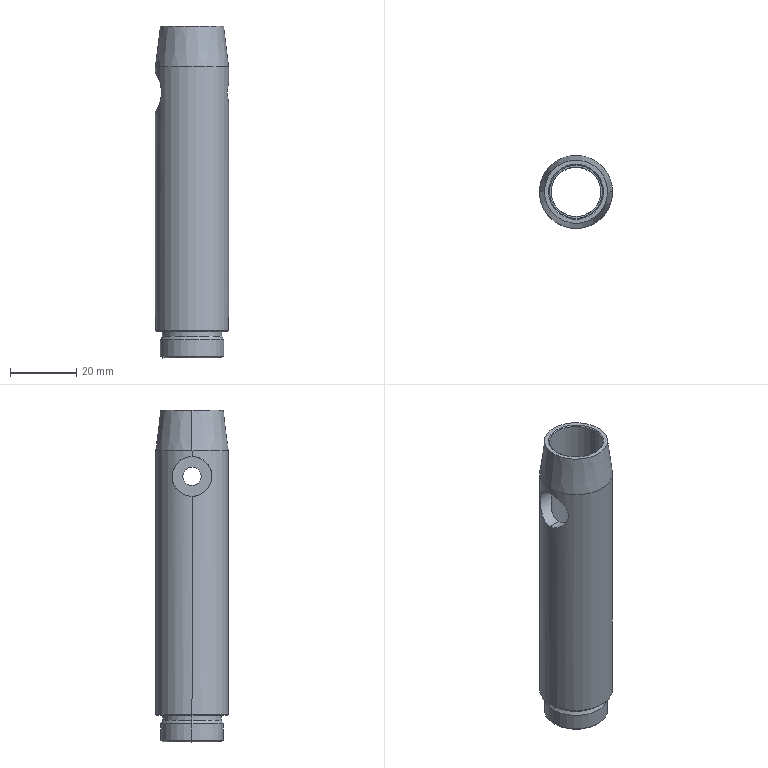Part | SolidWorks | features BaseBody 1 | 1 solid | 36 faces | box 22 x 22 x 100 mm | volume 17628 mm3 | cylinder 18 | cone 12 | plane 6 | commonest cylinder face diameters 12.01 x4 16 x4 5.5 x2 15 x2 17.8 x2 19 x2
STEP:
#1=CARTESIAN_POINT('',(469.537,37.715,-6.334));
#2=VERTEX_POINT('',#1);
#3=CARTESIAN_POINT('',(491.537,37.715,-6.334));
#4=VERTEX_POINT('',#3);
#5=CARTESIAN_POINT('',(480.537,37.715,-6.334));
#6=DIRECTION('',(0.000000013,0.,-1.));
#7=DIRECTION('',(0.,1.,0.));
#8=AXIS2_PLACEMENT_3D('',#5,#6,#7);
#9=CIRCLE('',#8,11.);
#10=EDGE_CURVE('',#2,#4,#9,.T.);
#11=ORIENTED_EDGE('',*,*,#10,.F.);
#12=CARTESIAN_POINT('',(469.537,37.715,59.361));
#13=VERTEX_POINT('',#12);
#14=CARTESIAN_POINT('',(469.537,37.715,-6.334));
#15=DIRECTION('',(-0.000000013,0.,1.));
#16=VECTOR('',#15,1000.);
#17=LINE('',#14,#16);
#18=EDGE_CURVE('',#2,#13,#17,.T.);
#19=ORIENTED_EDGE('',*,*,#18,.T.);
#20=CARTESIAN_POINT('',(469.537,37.715,71.371));
#21=VERTEX_POINT('',#20);
#22=CARTESIAN_POINT('',(469.537,37.715,71.371));
#23=CARTESIAN_POINT('',(469.537,37.916,71.371));
#24=CARTESIAN_POINT('',(469.542,38.12,71.361));
#25=CARTESIAN_POINT('',(469.565,38.52,71.32));
#26=CARTESIAN_POINT('',(469.581,38.717,71.29));
#27=CARTESIAN_POINT('',(469.624,39.107,71.211));
#28=CARTESIAN_POINT('',(469.65,39.3,71.161));
#29=CARTESIAN_POINT('',(469.712,39.68,71.044));
#30=CARTESIAN_POINT('',(469.748,39.868,70.975));
#31=CARTESIAN_POINT('',(469.867,40.414,70.745));
#32=CARTESIAN_POINT('',(469.96,40.756,70.558));
#33=CARTESIAN_POINT('',(470.116,41.24,70.231));
#34=CARTESIAN_POINT('',(470.17,41.397,70.114));
#35=CARTESIAN_POINT('',(470.281,41.695,69.866));
#36=CARTESIAN_POINT('',(470.337,41.837,69.737));
#37=CARTESIAN_POINT('',(470.508,42.243,69.328));
#38=CARTESIAN_POINT('',(470.624,42.488,69.03));
#39=CARTESIAN_POINT('',(470.844,42.921,68.383));
#40=CARTESIAN_POINT('',(470.946,43.104,68.043));
#41=CARTESIAN_POINT('',(471.077,43.33,67.504));
#42=CARTESIAN_POINT('',(471.118,43.396,67.32));
#43=CARTESIAN_POINT('',(471.189,43.513,66.941));
#44=CARTESIAN_POINT('',(471.22,43.562,66.746));
#45=CARTESIAN_POINT('',(471.295,43.681,66.157));
#46=CARTESIAN_POINT('',(471.321,43.721,65.756));
#47=CARTESIAN_POINT('',(471.32,43.719,64.946));
#48=CARTESIAN_POINT('',(471.292,43.677,64.549));
#49=CARTESIAN_POINT('',(471.192,43.518,63.772));
#50=CARTESIAN_POINT('',(471.117,43.398,63.389));
#51=CARTESIAN_POINT('',(470.94,43.094,62.669));
#52=CARTESIAN_POINT('',(470.838,42.909,62.328));
#53=CARTESIAN_POINT('',(470.617,42.474,61.684));
#54=CARTESIAN_POINT('',(470.502,42.229,61.387));
#55=CARTESIAN_POINT('',(470.331,41.822,60.981));
#56=CARTESIAN_POINT('',(470.275,41.68,60.852));
#57=CARTESIAN_POINT('',(470.165,41.381,60.606));
#58=CARTESIAN_POINT('',(470.11,41.224,60.489));
#59=CARTESIAN_POINT('',(469.956,40.741,60.165));
#60=CARTESIAN_POINT('',(469.863,40.4,59.981));
#61=CARTESIAN_POINT('',(469.707,39.678,59.678));
#62=CARTESIAN_POINT('',(469.643,39.292,59.558));
#63=CARTESIAN_POINT('',(469.559,38.512,59.401));
#64=CARTESIAN_POINT('',(469.537,38.117,59.361));
#65=CARTESIAN_POINT('',(469.537,37.715,59.361));
#66=B_SPLINE_CURVE_WITH_KNOTS('',3,(#22,#23,#24,#25,#26,#27,#28,#29,#30,#31,#32,#33,#34,#35,#36,#37,#38,#39,#40,#41,#42,#43,#44,#45,#46,#47,#48,#49,#50,#51,#52,#53,#54,#55,#56,#57,#58,#59,#60,#61,#62,#63,#64,#65),.UNSPECIFIED.,.F.,.F.,(4,2,2,2,2,2,2,2,2,2,2,2,2,2,2,2,2,2,2,2,2,4),(0.02874,0.02934,0.02994,0.03054,0.03113,0.03233,0.03293,0.03353,0.03472,0.03592,0.03652,0.03712,0.03832,0.03951,0.04071,0.04191,0.0431,0.0437,0.0443,0.0455,0.04669,0.04789),.UNSPECIFIED.);
#67=EDGE_CURVE('',#21,#13,#66,.T.);
#68=ORIENTED_EDGE('',*,*,#67,.F.);
#69=CARTESIAN_POINT('',(469.537,37.715,73.266));
#70=VERTEX_POINT('',#69);
#71=CARTESIAN_POINT('',(469.537,37.715,-6.334));
#72=DIRECTION('',(-0.000000013,0.,1.));
#73=VECTOR('',#72,1000.);
#74=LINE('',#71,#73);
#75=EDGE_CURVE('',#21,#70,#74,.T.);
#76=ORIENTED_EDGE('',*,*,#75,.T.);
#77=CARTESIAN_POINT('',(491.537,37.715,73.266));
#78=VERTEX_POINT('',#77);
#79=CARTESIAN_POINT('',(480.537,37.715,73.266));
#80=DIRECTION('',(-0.000000013,0.,1.));
#81=DIRECTION('',(0.,1.,0.));
#82=AXIS2_PLACEMENT_3D('',#79,#80,#81);
#83=CIRCLE('',#82,11.);
#84=EDGE_CURVE('',#78,#70,#83,.T.);
#85=ORIENTED_EDGE('',*,*,#84,.F.);
#86=CARTESIAN_POINT('',(491.537,37.715,68.116));
#87=VERTEX_POINT('',#86);
#88=CARTESIAN_POINT('',(491.537,37.715,-6.334));
#89=DIRECTION('',(-0.000000013,0.,1.));
#90=VECTOR('',#89,1000.);
#91=LINE('',#88,#90);
#92=EDGE_CURVE('',#87,#78,#91,.T.);
#93=ORIENTED_EDGE('',*,*,#92,.F.);
#94=CARTESIAN_POINT('',(491.537,37.715,62.616));
#95=VERTEX_POINT('',#94);
#96=CARTESIAN_POINT('',(491.537,37.715,62.616));
#97=CARTESIAN_POINT('',(491.537,37.895,62.616));
#98=CARTESIAN_POINT('',(491.532,38.078,62.634));
#99=CARTESIAN_POINT('',(491.515,38.431,62.705));
#100=CARTESIAN_POINT('',(491.502,38.603,62.757));
#101=CARTESIAN_POINT('',(491.454,39.103,62.965));
#102=CARTESIAN_POINT('',(491.409,39.406,63.167));
#103=CARTESIAN_POINT('',(491.341,39.787,63.55));
#104=CARTESIAN_POINT('',(491.318,39.901,63.688));
#105=CARTESIAN_POINT('',(491.276,40.1,63.985));
#106=CARTESIAN_POINT('',(491.256,40.186,64.146));
#107=CARTESIAN_POINT('',(491.223,40.324,64.478));
#108=CARTESIAN_POINT('',(491.21,40.376,64.649));
#109=CARTESIAN_POINT('',(491.192,40.447,65.003));
#110=CARTESIAN_POINT('',(491.188,40.465,65.186));
#111=CARTESIAN_POINT('',(491.188,40.465,65.551));
#112=CARTESIAN_POINT('',(491.192,40.446,65.73));
#113=CARTESIAN_POINT('',(491.21,40.376,66.082));
#114=CARTESIAN_POINT('',(491.224,40.322,66.257));
#115=CARTESIAN_POINT('',(491.256,40.184,66.59));
#116=CARTESIAN_POINT('',(491.276,40.099,66.747));
#117=CARTESIAN_POINT('',(491.318,39.9,67.045));
#118=CARTESIAN_POINT('',(491.341,39.784,67.186));
#119=CARTESIAN_POINT('',(491.409,39.405,67.564));
#120=CARTESIAN_POINT('',(491.454,39.099,67.769));
#121=CARTESIAN_POINT('',(491.502,38.603,67.975));
#122=CARTESIAN_POINT('',(491.515,38.429,68.028));
#123=CARTESIAN_POINT('',(491.532,38.074,68.098));
#124=CARTESIAN_POINT('',(491.537,37.895,68.116));
#125=CARTESIAN_POINT('',(491.537,37.715,68.116));
#126=B_SPLINE_CURVE_WITH_KNOTS('',3,(#96,#97,#98,#99,#100,#101,#102,#103,#104,#105,#106,#107,#108,#109,#110,#111,#112,#113,#114,#115,#116,#117,#118,#119,#120,#121,#122,#123,#124,#125),.UNSPECIFIED.,.F.,.F.,(4,2,2,2,2,2,2,2,2,2,2,2,2,2,4),(0.004317,0.004856,0.005396,0.006474,0.007014,0.007553,0.008092,0.008632,0.009171,0.00971,0.01025,0.01079,0.01187,0.01241,0.01295),.UNSPECIFIED.);
#127=EDGE_CURVE('',#95,#87,#126,.T.);
#128=ORIENTED_EDGE('',*,*,#127,.F.);
#129=CARTESIAN_POINT('',(491.537,37.715,-6.334));
#130=DIRECTION('',(-0.000000013,0.,1.));
#131=VECTOR('',#130,1000.);
#132=LINE('',#129,#131);
#133=EDGE_CURVE('',#4,#95,#132,.T.);
#134=ORIENTED_EDGE('',*,*,#133,.F.);
#135=EDGE_LOOP('',(#11,#19,#68,#76,#85,#93,#128,#134));
#136=FACE_OUTER_BOUND('',#135,.T.);
#137=CARTESIAN_POINT('',(480.537,37.715,-6.334));
#138=DIRECTION('',(-0.000000013,0.,1.));
#139=DIRECTION('',(1.,0.,0.000000013));
#140=AXIS2_PLACEMENT_3D('',#137,#138,#139);
#141=CYLINDRICAL_SURFACE('',#140,11.);
#142=ADVANCED_FACE('',(#136),#141,.T.);
#143=CARTESIAN_POINT('',(469.837,37.715,-6.634));
#144=VERTEX_POINT('',#143);
#145=CARTESIAN_POINT('',(491.237,37.715,-6.634));
#146=VERTEX_POINT('',#145);
#147=CARTESIAN_POINT('',(480.537,37.715,-6.634));
#148=DIRECTION('',(0.000000013,0.,-1.));
#149=DIRECTION('',(1.,0.,0.000000013));
#150=AXIS2_PLACEMENT_3D('',#147,#148,#149);
#151=CIRCLE('',#150,10.7);
#152=EDGE_CURVE('',#144,#146,#151,.T.);
#153=ORIENTED_EDGE('',*,*,#152,.F.);
#154=CARTESIAN_POINT('',(469.837,37.715,-6.634));
#155=DIRECTION('',(-0.7071,0.,0.7071));
#156=VECTOR('',#155,1000.);
#157=LINE('',#154,#156);
#158=EDGE_CURVE('',#144,#2,#157,.T.);
#159=ORIENTED_EDGE('',*,*,#158,.T.);
#160=ORIENTED_EDGE('',*,*,#10,.T.);
#161=CARTESIAN_POINT('',(491.237,37.715,-6.634));
#162=DIRECTION('',(0.7071,0.,0.7071));
#163=VECTOR('',#162,1000.);
#164=LINE('',#161,#163);
#165=EDGE_CURVE('',#146,#4,#164,.T.);
#166=ORIENTED_EDGE('',*,*,#165,.F.);
#167=EDGE_LOOP('',(#153,#159,#160,#166));
#168=FACE_OUTER_BOUND('',#167,.T.);
#169=CARTESIAN_POINT('',(480.537,37.715,-6.634));
#170=DIRECTION('',(-0.000000013,0.,1.));
#171=DIRECTION('',(1.,0.,0.000000013));
#172=AXIS2_PLACEMENT_3D('',#169,#170,#171);
#173=CONICAL_SURFACE('',#172,10.7,0.7854);
#174=ADVANCED_FACE('',(#168),#173,.T.);
#175=CARTESIAN_POINT('',(490.037,37.715,85.366));
#176=VERTEX_POINT('',#175);
#177=CARTESIAN_POINT('',(471.037,37.715,85.366));
#178=VERTEX_POINT('',#177);
#179=CARTESIAN_POINT('',(480.537,37.715,85.366));
#180=DIRECTION('',(-0.000000013,0.,1.));
#181=DIRECTION('',(-1.,0.,-0.000000013));
#182=AXIS2_PLACEMENT_3D('',#179,#180,#181);
#183=CIRCLE('',#182,9.5);
#184=EDGE_CURVE('',#176,#178,#183,.T.);
#185=ORIENTED_EDGE('',*,*,#184,.F.);
#186=CARTESIAN_POINT('',(491.537,37.715,73.266));
#187=DIRECTION('',(0.123,0.,-0.9924));
#188=VECTOR('',#187,1000.);
#189=LINE('',#186,#188);
#190=EDGE_CURVE('',#176,#78,#189,.T.);
#191=ORIENTED_EDGE('',*,*,#190,.T.);
#192=ORIENTED_EDGE('',*,*,#84,.T.);
#193=CARTESIAN_POINT('',(469.537,37.715,73.266));
#194=DIRECTION('',(-0.123,0.,-0.9924));
#195=VECTOR('',#194,1000.);
#196=LINE('',#193,#195);
#197=EDGE_CURVE('',#178,#70,#196,.T.);
#198=ORIENTED_EDGE('',*,*,#197,.F.);
#199=EDGE_LOOP('',(#185,#191,#192,#198));
#200=FACE_OUTER_BOUND('',#199,.T.);
#201=CARTESIAN_POINT('',(480.537,37.715,73.266));
#202=DIRECTION('',(0.000000013,0.,-1.));
#203=DIRECTION('',(-1.,0.,-0.000000013));
#204=AXIS2_PLACEMENT_3D('',#201,#202,#203);
#205=CONICAL_SURFACE('',#204,11.,0.1233);
#206=ADVANCED_FACE('',(#200),#205,.T.);
#207=CARTESIAN_POINT('',(491.537,37.715,68.116));
#208=CARTESIAN_POINT('',(491.537,37.535,68.116));
#209=CARTESIAN_POINT('',(491.532,37.352,68.098));
#210=CARTESIAN_POINT('',(491.515,36.998,68.027));
#211=CARTESIAN_POINT('',(491.502,36.827,67.975));
#212=CARTESIAN_POINT('',(491.454,36.326,67.767));
#213=CARTESIAN_POINT('',(491.409,36.024,67.564));
#214=CARTESIAN_POINT('',(491.341,35.642,67.182));
#215=CARTESIAN_POINT('',(491.318,35.529,67.044));
#216=CARTESIAN_POINT('',(491.276,35.33,66.747));
#217=CARTESIAN_POINT('',(491.256,35.244,66.586));
#218=CARTESIAN_POINT('',(491.223,35.106,66.254));
#219=CARTESIAN_POINT('',(491.21,35.054,66.083));
#220=CARTESIAN_POINT('',(491.192,34.983,65.728));
#221=CARTESIAN_POINT('',(491.188,34.965,65.546));
#222=CARTESIAN_POINT('',(491.188,34.965,65.181));
#223=CARTESIAN_POINT('',(491.192,34.983,65.002));
#224=CARTESIAN_POINT('',(491.21,35.054,64.65));
#225=CARTESIAN_POINT('',(491.224,35.107,64.475));
#226=CARTESIAN_POINT('',(491.256,35.245,64.142));
#227=CARTESIAN_POINT('',(491.276,35.33,63.985));
#228=CARTESIAN_POINT('',(491.318,35.53,63.686));
#229=CARTESIAN_POINT('',(491.341,35.646,63.546));
#230=CARTESIAN_POINT('',(491.409,36.025,63.167));
#231=CARTESIAN_POINT('',(491.454,36.33,62.963));
#232=CARTESIAN_POINT('',(491.502,36.826,62.757));
#233=CARTESIAN_POINT('',(491.515,37.,62.704));
#234=CARTESIAN_POINT('',(491.532,37.356,62.633));
#235=CARTESIAN_POINT('',(491.537,37.535,62.616));
#236=CARTESIAN_POINT('',(491.537,37.715,62.616));
#237=B_SPLINE_CURVE_WITH_KNOTS('',3,(#207,#208,#209,#210,#211,#212,#213,#214,#215,#216,#217,#218,#219,#220,#221,#222,#223,#224,#225,#226,#227,#228,#229,#230,#231,#232,#233,#234,#235,#236),.UNSPECIFIED.,.F.,.F.,(4,2,2,2,2,2,2,2,2,2,2,2,2,2,4),(0.01295,0.01349,0.01403,0.0151,0.01564,0.01618,0.01672,0.01726,0.0178,0.01834,0.01888,0.01942,0.0205,0.02104,0.02158),.UNSPECIFIED.);
#238=EDGE_CURVE('',#87,#95,#237,.T.);
#239=ORIENTED_EDGE('',*,*,#238,.T.);
#240=CARTESIAN_POINT('',(489.037,37.715,62.616));
#241=VERTEX_POINT('',#240);
#242=CARTESIAN_POINT('',(491.552,37.715,62.616));
#243=DIRECTION('',(-1.,0.,-0.000000013));
#244=VECTOR('',#243,1000.);
#245=LINE('',#242,#244);
#246=EDGE_CURVE('',#95,#241,#245,.T.);
#247=ORIENTED_EDGE('',*,*,#246,.T.);
#248=CARTESIAN_POINT('',(489.037,37.715,68.116));
#249=VERTEX_POINT('',#248);
#250=CARTESIAN_POINT('',(489.037,37.715,65.366));
#251=DIRECTION('',(-1.,0.,-0.000000013));
#252=DIRECTION('',(-0.000000013,0.,1.));
#253=AXIS2_PLACEMENT_3D('',#250,#251,#252);
#254=CIRCLE('',#253,2.75);
#255=EDGE_CURVE('',#241,#249,#254,.T.);
#256=ORIENTED_EDGE('',*,*,#255,.T.);
#257=CARTESIAN_POINT('',(491.552,37.715,68.116));
#258=DIRECTION('',(-1.,0.,-0.000000013));
#259=VECTOR('',#258,1000.);
#260=LINE('',#257,#259);
#261=EDGE_CURVE('',#87,#249,#260,.T.);
#262=ORIENTED_EDGE('',*,*,#261,.F.);
#263=EDGE_LOOP('',(#239,#247,#256,#262));
#264=FACE_OUTER_BOUND('',#263,.T.);
#265=CARTESIAN_POINT('',(491.552,37.715,65.366));
#266=DIRECTION('',(-1.,0.,-0.000000013));
#267=DIRECTION('',(-0.000000013,0.,1.));
#268=AXIS2_PLACEMENT_3D('',#265,#266,#267);
#269=CYLINDRICAL_SURFACE('',#268,2.75);
#270=ADVANCED_FACE('',(#264),#269,.F.);
#271=CARTESIAN_POINT('',(469.537,37.715,59.361));
#272=CARTESIAN_POINT('',(469.537,37.514,59.361));
#273=CARTESIAN_POINT('',(469.542,37.31,59.371));
#274=CARTESIAN_POINT('',(469.564,36.911,59.412));
#275=CARTESIAN_POINT('',(469.581,36.713,59.442));
#276=CARTESIAN_POINT('',(469.623,36.324,59.521));
#277=CARTESIAN_POINT('',(469.65,36.131,59.57));
#278=CARTESIAN_POINT('',(469.712,35.752,59.687));
#279=CARTESIAN_POINT('',(469.748,35.563,59.756));
#280=CARTESIAN_POINT('',(469.866,35.018,59.986));
#281=CARTESIAN_POINT('',(469.96,34.676,60.172));
#282=CARTESIAN_POINT('',(470.115,34.192,60.499));
#283=CARTESIAN_POINT('',(470.169,34.036,60.616));
#284=CARTESIAN_POINT('',(470.28,33.737,60.863));
#285=CARTESIAN_POINT('',(470.336,33.595,60.992));
#286=CARTESIAN_POINT('',(470.507,33.189,61.4));
#287=CARTESIAN_POINT('',(470.622,32.944,61.698));
#288=CARTESIAN_POINT('',(470.842,32.511,62.344));
#289=CARTESIAN_POINT('',(470.944,32.328,62.684));
#290=CARTESIAN_POINT('',(471.076,32.102,63.221));
#291=CARTESIAN_POINT('',(471.116,32.035,63.405));
#292=CARTESIAN_POINT('',(471.187,31.919,63.783));
#293=CARTESIAN_POINT('',(471.219,31.869,63.978));
#294=CARTESIAN_POINT('',(471.294,31.75,64.566));
#295=CARTESIAN_POINT('',(471.321,31.709,64.965));
#296=CARTESIAN_POINT('',(471.32,31.71,65.777));
#297=CARTESIAN_POINT('',(471.293,31.751,66.174));
#298=CARTESIAN_POINT('',(471.193,31.909,66.952));
#299=CARTESIAN_POINT('',(471.119,32.029,67.336));
#300=CARTESIAN_POINT('',(470.942,32.332,68.057));
#301=CARTESIAN_POINT('',(470.839,32.517,68.398));
#302=CARTESIAN_POINT('',(470.619,32.952,69.044));
#303=CARTESIAN_POINT('',(470.503,33.197,69.341));
#304=CARTESIAN_POINT('',(470.333,33.604,69.748));
#305=CARTESIAN_POINT('',(470.276,33.747,69.877));
#306=CARTESIAN_POINT('',(470.166,34.045,70.123));
#307=CARTESIAN_POINT('',(470.111,34.202,70.241));
#308=CARTESIAN_POINT('',(469.957,34.686,70.566));
#309=CARTESIAN_POINT('',(469.864,35.027,70.75));
#310=CARTESIAN_POINT('',(469.708,35.749,71.054));
#311=CARTESIAN_POINT('',(469.644,36.136,71.173));
#312=CARTESIAN_POINT('',(469.559,36.916,71.331));
#313=CARTESIAN_POINT('',(469.537,37.312,71.371));
#314=CARTESIAN_POINT('',(469.537,37.715,71.371));
#315=B_SPLINE_CURVE_WITH_KNOTS('',3,(#271,#272,#273,#274,#275,#276,#277,#278,#279,#280,#281,#282,#283,#284,#285,#286,#287,#288,#289,#290,#291,#292,#293,#294,#295,#296,#297,#298,#299,#300,#301,#302,#303,#304,#305,#306,#307,#308,#309,#310,#311,#312,#313,#314),.UNSPECIFIED.,.F.,.F.,(4,2,2,2,2,2,2,2,2,2,2,2,2,2,2,2,2,2,2,2,2,4),(0.00959,0.01019,0.01079,0.01139,0.01198,0.01318,0.01378,0.01438,0.01557,0.01677,0.01737,0.01797,0.01917,0.02036,0.02156,0.02276,0.02395,0.02455,0.02515,0.02635,0.02754,0.02874),.UNSPECIFIED.);
#316=EDGE_CURVE('',#13,#21,#315,.T.);
#317=ORIENTED_EDGE('',*,*,#316,.T.);
#318=CARTESIAN_POINT('',(473.037,37.715,71.371));
#319=VERTEX_POINT('',#318);
#320=CARTESIAN_POINT('',(469.498,37.715,71.371));
#321=DIRECTION('',(1.,0.,0.000000013));
#322=VECTOR('',#321,1000.);
#323=LINE('',#320,#322);
#324=EDGE_CURVE('',#21,#319,#323,.T.);
#325=ORIENTED_EDGE('',*,*,#324,.T.);
#326=CARTESIAN_POINT('',(473.037,37.715,59.361));
#327=VERTEX_POINT('',#326);
#328=CARTESIAN_POINT('',(473.037,37.715,71.371));
#329=CARTESIAN_POINT('',(473.037,37.507,71.371));
#330=CARTESIAN_POINT('',(473.045,37.3,71.36));
#331=CARTESIAN_POINT('',(473.08,36.888,71.317));
#332=CARTESIAN_POINT('',(473.106,36.68,71.285));
#333=CARTESIAN_POINT('',(473.207,36.074,71.157));
#334=CARTESIAN_POINT('',(473.305,35.689,71.033));
#335=CARTESIAN_POINT('',(473.491,35.138,70.794));
#336=CARTESIAN_POINT('',(473.559,34.959,70.705));
#337=CARTESIAN_POINT('',(473.704,34.617,70.514));
#338=CARTESIAN_POINT('',(473.781,34.453,70.412));
#339=CARTESIAN_POINT('',(474.023,33.98,70.084));
#340=CARTESIAN_POINT('',(474.202,33.687,69.836));
#341=CARTESIAN_POINT('',(474.567,33.163,69.301));
#342=CARTESIAN_POINT('',(474.755,32.929,69.013));
#343=CARTESIAN_POINT('',(475.127,32.513,68.39));
#344=CARTESIAN_POINT('',(475.309,32.333,68.057));
#345=CARTESIAN_POINT('',(475.553,32.109,67.528));
#346=CARTESIAN_POINT('',(475.629,32.042,67.347));
#347=CARTESIAN_POINT('',(475.769,31.925,66.97));
#348=CARTESIAN_POINT('',(475.832,31.874,66.774));
#349=CARTESIAN_POINT('',(475.986,31.752,66.181));
#350=CARTESIAN_POINT('',(476.045,31.709,65.771));
#351=CARTESIAN_POINT('',(476.042,31.711,64.929));
#352=CARTESIAN_POINT('',(475.981,31.756,64.521));
#353=CARTESIAN_POINT('',(475.822,31.881,63.926));
#354=CARTESIAN_POINT('',(475.759,31.933,63.732));
#355=CARTESIAN_POINT('',(475.619,32.051,63.36));
#356=CARTESIAN_POINT('',(475.542,32.119,63.18));
#357=CARTESIAN_POINT('',(475.297,32.344,62.653));
#358=CARTESIAN_POINT('',(475.114,32.526,62.32));
#359=CARTESIAN_POINT('',(474.746,32.941,61.704));
#360=CARTESIAN_POINT('',(474.559,33.174,61.419));
#361=CARTESIAN_POINT('',(474.196,33.697,60.888));
#362=CARTESIAN_POINT('',(474.018,33.989,60.641));
#363=CARTESIAN_POINT('',(473.696,34.619,60.206));
#364=CARTESIAN_POINT('',(473.552,34.957,60.017));
#365=CARTESIAN_POINT('',(473.367,35.506,59.778));
#366=CARTESIAN_POINT('',(473.311,35.696,59.707));
#367=CARTESIAN_POINT('',(473.214,36.082,59.584));
#368=CARTESIAN_POINT('',(473.173,36.278,59.532));
#369=CARTESIAN_POINT('',(473.073,36.879,59.405));
#370=CARTESIAN_POINT('',(473.037,37.3,59.361));
#371=CARTESIAN_POINT('',(473.037,37.715,59.361));
#372=B_SPLINE_CURVE_WITH_KNOTS('',3,(#328,#329,#330,#331,#332,#333,#334,#335,#336,#337,#338,#339,#340,#341,#342,#343,#344,#345,#346,#347,#348,#349,#350,#351,#352,#353,#354,#355,#356,#357,#358,#359,#360,#361,#362,#363,#364,#365,#366,#367,#368,#369,#370,#371),.UNSPECIFIED.,.F.,.F.,(4,2,2,2,2,2,2,2,2,2,2,2,2,2,2,2,2,2,2,2,2,4),(0.02988,0.0305,0.03112,0.03237,0.03299,0.03361,0.03485,0.0361,0.03734,0.03796,0.03859,0.03983,0.04107,0.0417,0.04232,0.04356,0.04481,0.04605,0.0473,0.04792,0.04854,0.04978),.UNSPECIFIED.);
#373=EDGE_CURVE('',#319,#327,#372,.T.);
#374=ORIENTED_EDGE('',*,*,#373,.T.);
#375=CARTESIAN_POINT('',(469.498,37.715,59.361));
#376=DIRECTION('',(1.,0.,0.000000013));
#377=VECTOR('',#376,1000.);
#378=LINE('',#375,#377);
#379=EDGE_CURVE('',#13,#327,#378,.T.);
#380=ORIENTED_EDGE('',*,*,#379,.F.);
#381=EDGE_LOOP('',(#317,#325,#374,#380));
#382=FACE_OUTER_BOUND('',#381,.T.);
#383=CARTESIAN_POINT('',(469.498,37.715,65.366));
#384=DIRECTION('',(1.,0.,0.000000013));
#385=DIRECTION('',(0.000000013,0.,-1.));
#386=AXIS2_PLACEMENT_3D('',#383,#384,#385);
#387=CYLINDRICAL_SURFACE('',#386,6.005);
#388=ADVANCED_FACE('',(#382),#387,.F.);
#389=CARTESIAN_POINT('',(488.037,37.715,-2.634));
#390=VERTEX_POINT('',#389);
#391=CARTESIAN_POINT('',(473.037,37.715,-2.634));
#392=VERTEX_POINT('',#391);
#393=CARTESIAN_POINT('',(480.537,37.715,-2.634));
#394=DIRECTION('',(0.000000013,0.,-1.));
#395=DIRECTION('',(1.,0.,0.000000013));
#396=AXIS2_PLACEMENT_3D('',#393,#394,#395);
#397=CIRCLE('',#396,7.5);
#398=EDGE_CURVE('',#390,#392,#397,.T.);
#399=ORIENTED_EDGE('',*,*,#398,.T.);
#400=CARTESIAN_POINT('',(473.037,37.715,-2.634));
#401=DIRECTION('',(-0.000000013,0.,1.));
#402=VECTOR('',#401,1000.);
#403=LINE('',#400,#402);
#404=EDGE_CURVE('',#392,#327,#403,.T.);
#405=ORIENTED_EDGE('',*,*,#404,.T.);
#406=ORIENTED_EDGE('',*,*,#373,.F.);
#407=CARTESIAN_POINT('',(473.037,37.715,73.366));
#408=VERTEX_POINT('',#407);
#409=CARTESIAN_POINT('',(473.037,37.715,-2.634));
#410=DIRECTION('',(-0.000000013,0.,1.));
#411=VECTOR('',#410,1000.);
#412=LINE('',#409,#411);
#413=EDGE_CURVE('',#319,#408,#412,.T.);
#414=ORIENTED_EDGE('',*,*,#413,.T.);
#415=CARTESIAN_POINT('',(488.037,37.715,73.366));
#416=VERTEX_POINT('',#415);
#417=CARTESIAN_POINT('',(480.537,37.715,73.366));
#418=DIRECTION('',(-0.000000013,0.,1.));
#419=DIRECTION('',(1.,0.,0.000000013));
#420=AXIS2_PLACEMENT_3D('',#417,#418,#419);
#421=CIRCLE('',#420,7.5);
#422=EDGE_CURVE('',#408,#416,#421,.T.);
#423=ORIENTED_EDGE('',*,*,#422,.T.);
#424=CARTESIAN_POINT('',(488.037,37.715,71.371));
#425=VERTEX_POINT('',#424);
#426=CARTESIAN_POINT('',(488.037,37.715,-2.634));
#427=DIRECTION('',(-0.000000013,0.,1.));
#428=VECTOR('',#427,1000.);
#429=LINE('',#426,#428);
#430=EDGE_CURVE('',#425,#416,#429,.T.);
#431=ORIENTED_EDGE('',*,*,#430,.F.);
#432=CARTESIAN_POINT('',(488.037,37.715,59.361));
#433=VERTEX_POINT('',#432);
#434=CARTESIAN_POINT('',(488.037,37.715,59.361));
#435=CARTESIAN_POINT('',(488.037,37.508,59.361));
#436=CARTESIAN_POINT('',(488.028,37.301,59.372));
#437=CARTESIAN_POINT('',(487.994,36.889,59.414));
#438=CARTESIAN_POINT('',(487.968,36.682,59.447));
#439=CARTESIAN_POINT('',(487.867,36.077,59.574));
#440=CARTESIAN_POINT('',(487.769,35.692,59.698));
#441=CARTESIAN_POINT('',(487.584,35.142,59.936));
#442=CARTESIAN_POINT('',(487.517,34.964,60.025));
#443=CARTESIAN_POINT('',(487.372,34.623,60.215));
#444=CARTESIAN_POINT('',(487.296,34.459,60.317));
#445=CARTESIAN_POINT('',(487.054,33.986,60.644));
#446=CARTESIAN_POINT('',(486.876,33.693,60.891));
#447=CARTESIAN_POINT('',(486.511,33.169,61.424));
#448=CARTESIAN_POINT('',(486.324,32.936,61.711));
#449=CARTESIAN_POINT('',(485.953,32.519,62.332));
#450=CARTESIAN_POINT('',(485.771,32.338,62.664));
#451=CARTESIAN_POINT('',(485.526,32.114,63.191));
#452=CARTESIAN_POINT('',(485.45,32.047,63.372));
#453=CARTESIAN_POINT('',(485.31,31.929,63.747));
#454=CARTESIAN_POINT('',(485.247,31.877,63.942));
#455=CARTESIAN_POINT('',(485.091,31.754,64.533));
#456=CARTESIAN_POINT('',(485.031,31.71,64.94));
#457=CARTESIAN_POINT('',(485.03,31.709,65.785));
#458=CARTESIAN_POINT('',(485.09,31.753,66.194));
#459=CARTESIAN_POINT('',(485.247,31.878,66.791));
#460=CARTESIAN_POINT('',(485.31,31.929,66.985));
#461=CARTESIAN_POINT('',(485.449,32.047,67.359));
#462=CARTESIAN_POINT('',(485.526,32.114,67.54));
#463=CARTESIAN_POINT('',(485.77,32.338,68.067));
#464=CARTESIAN_POINT('',(485.954,32.52,68.402));
#465=CARTESIAN_POINT('',(486.323,32.935,69.02));
#466=CARTESIAN_POINT('',(486.51,33.168,69.306));
#467=CARTESIAN_POINT('',(486.874,33.691,69.839));
#468=CARTESIAN_POINT('',(487.052,33.983,70.086));
#469=CARTESIAN_POINT('',(487.375,34.614,70.523));
#470=CARTESIAN_POINT('',(487.52,34.952,70.713));
#471=CARTESIAN_POINT('',(487.706,35.502,70.952));
#472=CARTESIAN_POINT('',(487.762,35.693,71.024));
#473=CARTESIAN_POINT('',(487.859,36.079,71.147));
#474=CARTESIAN_POINT('',(487.9,36.275,71.2));
#475=CARTESIAN_POINT('',(488.001,36.877,71.326));
#476=CARTESIAN_POINT('',(488.037,37.3,71.371));
#477=CARTESIAN_POINT('',(488.037,37.715,71.371));
#478=B_SPLINE_CURVE_WITH_KNOTS('',3,(#434,#435,#436,#437,#438,#439,#440,#441,#442,#443,#444,#445,#446,#447,#448,#449,#450,#451,#452,#453,#454,#455,#456,#457,#458,#459,#460,#461,#462,#463,#464,#465,#466,#467,#468,#469,#470,#471,#472,#473,#474,#475,#476,#477),.UNSPECIFIED.,.F.,.F.,(4,2,2,2,2,2,2,2,2,2,2,2,2,2,2,2,2,2,2,2,2,4),(0.009969,0.01059,0.01121,0.01246,0.01308,0.0137,0.01495,0.01619,0.01743,0.01806,0.01868,0.01992,0.02117,0.02179,0.02241,0.02366,0.0249,0.02614,0.02739,0.02801,0.02863,0.02988),.UNSPECIFIED.);
#479=EDGE_CURVE('',#433,#425,#478,.T.);
#480=ORIENTED_EDGE('',*,*,#479,.F.);
#481=CARTESIAN_POINT('',(488.037,37.715,-2.634));
#482=DIRECTION('',(-0.000000013,0.,1.));
#483=VECTOR('',#482,1000.);
#484=LINE('',#481,#483);
#485=EDGE_CURVE('',#390,#433,#484,.T.);
#486=ORIENTED_EDGE('',*,*,#485,.F.);
#487=EDGE_LOOP('',(#399,#405,#406,#414,#423,#431,#480,#486));
#488=FACE_OUTER_BOUND('',#487,.T.);
#489=CARTESIAN_POINT('',(480.537,37.715,-2.634));
#490=DIRECTION('',(-0.000000013,0.,1.));
#491=DIRECTION('',(1.,0.,0.000000013));
#492=AXIS2_PLACEMENT_3D('',#489,#490,#491);
#493=CYLINDRICAL_SURFACE('',#492,7.5);
#494=ADVANCED_FACE('',(#488),#493,.F.);
#495=CARTESIAN_POINT('',(471.637,37.715,-8.134));
#496=VERTEX_POINT('',#495);
#497=CARTESIAN_POINT('',(489.437,37.715,-8.134));
#498=VERTEX_POINT('',#497);
#499=CARTESIAN_POINT('',(480.537,37.715,-8.134));
#500=DIRECTION('',(0.000000013,0.,-1.));
#501=DIRECTION('',(0.,1.,0.));
#502=AXIS2_PLACEMENT_3D('',#499,#500,#501);
#503=CIRCLE('',#502,8.9);
#504=EDGE_CURVE('',#496,#498,#503,.T.);
#505=ORIENTED_EDGE('',*,*,#504,.F.);
#506=CARTESIAN_POINT('',(471.637,37.715,-6.634));
#507=VERTEX_POINT('',#506);
#508=CARTESIAN_POINT('',(471.637,37.715,-8.134));
#509=DIRECTION('',(-0.000000013,0.,1.));
#510=VECTOR('',#509,1000.);
#511=LINE('',#508,#510);
#512=EDGE_CURVE('',#496,#507,#511,.T.);
#513=ORIENTED_EDGE('',*,*,#512,.T.);
#514=CARTESIAN_POINT('',(489.437,37.715,-6.634));
#515=VERTEX_POINT('',#514);
#516=CARTESIAN_POINT('',(480.537,37.715,-6.634));
#517=DIRECTION('',(0.000000013,0.,-1.));
#518=DIRECTION('',(1.,0.,0.000000013));
#519=AXIS2_PLACEMENT_3D('',#516,#517,#518);
#520=CIRCLE('',#519,8.9);
#521=EDGE_CURVE('',#507,#515,#520,.T.);
#522=ORIENTED_EDGE('',*,*,#521,.T.);
#523=CARTESIAN_POINT('',(489.437,37.715,-8.134));
#524=DIRECTION('',(-0.000000013,0.,1.));
#525=VECTOR('',#524,1000.);
#526=LINE('',#523,#525);
#527=EDGE_CURVE('',#498,#515,#526,.T.);
#528=ORIENTED_EDGE('',*,*,#527,.F.);
#529=EDGE_LOOP('',(#505,#513,#522,#528));
#530=FACE_OUTER_BOUND('',#529,.T.);
#531=CARTESIAN_POINT('',(480.537,37.715,-8.134));
#532=DIRECTION('',(-0.000000013,0.,1.));
#533=DIRECTION('',(1.,0.,0.000000013));
#534=AXIS2_PLACEMENT_3D('',#531,#532,#533);
#535=CYLINDRICAL_SURFACE('',#534,8.9);
#536=ADVANCED_FACE('',(#530),#535,.T.);
#537=CARTESIAN_POINT('',(488.537,37.715,85.066));
#538=VERTEX_POINT('',#537);
#539=CARTESIAN_POINT('',(472.537,37.715,85.066));
#540=VERTEX_POINT('',#539);
#541=CARTESIAN_POINT('',(480.537,37.715,85.066));
#542=DIRECTION('',(0.000000013,0.,-1.));
#543=DIRECTION('',(0.,1.,0.));
#544=AXIS2_PLACEMENT_3D('',#541,#542,#543);
#545=CIRCLE('',#544,8.);
#546=EDGE_CURVE('',#538,#540,#545,.T.);
#547=ORIENTED_EDGE('',*,*,#546,.T.);
#548=CARTESIAN_POINT('',(472.237,37.715,85.366));
#549=VERTEX_POINT('',#548);
#550=CARTESIAN_POINT('',(472.537,37.715,85.066));
#551=DIRECTION('',(-0.7071,0.,0.7071));
#552=VECTOR('',#551,1000.);
#553=LINE('',#550,#552);
#554=EDGE_CURVE('',#540,#549,#553,.T.);
#555=ORIENTED_EDGE('',*,*,#554,.T.);
#556=CARTESIAN_POINT('',(488.837,37.715,85.366));
#557=VERTEX_POINT('',#556);
#558=CARTESIAN_POINT('',(480.537,37.715,85.366));
#559=DIRECTION('',(0.000000013,0.,-1.));
#560=DIRECTION('',(1.,0.,0.000000013));
#561=AXIS2_PLACEMENT_3D('',#558,#559,#560);
#562=CIRCLE('',#561,8.3);
#563=EDGE_CURVE('',#557,#549,#562,.T.);
#564=ORIENTED_EDGE('',*,*,#563,.F.);
#565=CARTESIAN_POINT('',(488.537,37.715,85.066));
#566=DIRECTION('',(0.7071,0.,0.7071));
#567=VECTOR('',#566,1000.);
#568=LINE('',#565,#567);
#569=EDGE_CURVE('',#538,#557,#568,.T.);
#570=ORIENTED_EDGE('',*,*,#569,.F.);
#571=EDGE_LOOP('',(#547,#555,#564,#570));
#572=FACE_OUTER_BOUND('',#571,.T.);
#573=CARTESIAN_POINT('',(480.537,37.715,85.066));
#574=DIRECTION('',(-0.000000013,0.,1.));
#575=DIRECTION('',(1.,0.,0.000000013));
#576=AXIS2_PLACEMENT_3D('',#573,#574,#575);
#577=CONICAL_SURFACE('',#576,8.,0.7854);
#578=ADVANCED_FACE('',(#572),#577,.F.);
#579=ORIENTED_EDGE('',*,*,#479,.T.);
#580=CARTESIAN_POINT('',(489.037,37.715,71.371));
#581=VERTEX_POINT('',#580);
#582=CARTESIAN_POINT('',(485.006,37.715,71.371));
#583=DIRECTION('',(1.,0.,0.000000013));
#584=VECTOR('',#583,1000.);
#585=LINE('',#582,#584);
#586=EDGE_CURVE('',#425,#581,#585,.T.);
#587=ORIENTED_EDGE('',*,*,#586,.T.);
#588=CARTESIAN_POINT('',(489.037,37.715,59.361));
#589=VERTEX_POINT('',#588);
#590=CARTESIAN_POINT('',(489.037,37.715,65.366));
#591=DIRECTION('',(1.,0.,0.000000013));
#592=DIRECTION('',(0.000000013,0.,-1.));
#593=AXIS2_PLACEMENT_3D('',#590,#591,#592);
#594=CIRCLE('',#593,6.005);
#595=EDGE_CURVE('',#581,#589,#594,.T.);
#596=ORIENTED_EDGE('',*,*,#595,.T.);
#597=CARTESIAN_POINT('',(485.006,37.715,59.361));
#598=DIRECTION('',(1.,0.,0.000000013));
#599=VECTOR('',#598,1000.);
#600=LINE('',#597,#599);
#601=EDGE_CURVE('',#433,#589,#600,.T.);
#602=ORIENTED_EDGE('',*,*,#601,.F.);
#603=EDGE_LOOP('',(#579,#587,#596,#602));
#604=FACE_OUTER_BOUND('',#603,.T.);
#605=CARTESIAN_POINT('',(485.006,37.715,65.366));
#606=DIRECTION('',(1.,0.,0.000000013));
#607=DIRECTION('',(0.000000013,0.,-1.));
#608=AXIS2_PLACEMENT_3D('',#605,#606,#607);
#609=CYLINDRICAL_SURFACE('',#608,6.005);
#610=ADVANCED_FACE('',(#604),#609,.F.);
#611=ORIENTED_EDGE('',*,*,#504,.T.);
#612=CARTESIAN_POINT('',(490.037,37.715,-9.173));
#613=VERTEX_POINT('',#612);
#614=CARTESIAN_POINT('',(490.037,37.715,-9.173));
#615=DIRECTION('',(0.5,0.,-0.866));
#616=VECTOR('',#615,1000.);
#617=LINE('',#614,#616);
#618=EDGE_CURVE('',#498,#613,#617,.T.);
#619=ORIENTED_EDGE('',*,*,#618,.T.);
#620=CARTESIAN_POINT('',(471.037,37.715,-9.173));
#621=VERTEX_POINT('',#620);
#622=CARTESIAN_POINT('',(480.537,37.715,-9.173));
#623=DIRECTION('',(0.000000013,0.,-1.));
#624=DIRECTION('',(0.,1.,0.));
#625=AXIS2_PLACEMENT_3D('',#622,#623,#624);
#626=CIRCLE('',#625,9.5);
#627=EDGE_CURVE('',#621,#613,#626,.T.);
#628=ORIENTED_EDGE('',*,*,#627,.F.);
#629=CARTESIAN_POINT('',(471.037,37.715,-9.173));
#630=DIRECTION('',(-0.5,0.,-0.866));
#631=VECTOR('',#630,1000.);
#632=LINE('',#629,#631);
#633=EDGE_CURVE('',#496,#621,#632,.T.);
#634=ORIENTED_EDGE('',*,*,#633,.F.);
#635=EDGE_LOOP('',(#611,#619,#628,#634));
#636=FACE_OUTER_BOUND('',#635,.T.);
#637=CARTESIAN_POINT('',(480.537,37.715,-9.173));
#638=DIRECTION('',(0.000000013,0.,-1.));
#639=DIRECTION('',(-1.,0.,-0.000000013));
#640=AXIS2_PLACEMENT_3D('',#637,#638,#639);
#641=CONICAL_SURFACE('',#640,9.5,0.5236);
#642=ADVANCED_FACE('',(#636),#641,.T.);
#643=CARTESIAN_POINT('',(472.537,37.715,73.366));
#644=VERTEX_POINT('',#643);
#645=CARTESIAN_POINT('',(488.537,37.715,73.366));
#646=VERTEX_POINT('',#645);
#647=CARTESIAN_POINT('',(480.537,37.715,73.366));
#648=DIRECTION('',(-0.000000013,0.,1.));
#649=DIRECTION('',(1.,0.,0.000000013));
#650=AXIS2_PLACEMENT_3D('',#647,#648,#649);
#651=CIRCLE('',#650,8.);
#652=EDGE_CURVE('',#644,#646,#651,.T.);
#653=ORIENTED_EDGE('',*,*,#652,.F.);
#654=CARTESIAN_POINT('',(472.537,37.715,73.366));
#655=DIRECTION('',(-0.000000013,0.,1.));
#656=VECTOR('',#655,1000.);
#657=LINE('',#654,#656);
#658=EDGE_CURVE('',#644,#540,#657,.T.);
#659=ORIENTED_EDGE('',*,*,#658,.T.);
#660=ORIENTED_EDGE('',*,*,#546,.F.);
#661=CARTESIAN_POINT('',(488.537,37.715,73.366));
#662=DIRECTION('',(-0.000000013,0.,1.));
#663=VECTOR('',#662,1000.);
#664=LINE('',#661,#663);
#665=EDGE_CURVE('',#646,#538,#664,.T.);
#666=ORIENTED_EDGE('',*,*,#665,.F.);
#667=EDGE_LOOP('',(#653,#659,#660,#666));
#668=FACE_OUTER_BOUND('',#667,.T.);
#669=CARTESIAN_POINT('',(480.537,37.715,73.366));
#670=DIRECTION('',(-0.000000013,0.,1.));
#671=DIRECTION('',(1.,0.,0.000000013));
#672=AXIS2_PLACEMENT_3D('',#669,#670,#671);
#673=CYLINDRICAL_SURFACE('',#672,8.);
#674=ADVANCED_FACE('',(#668),#673,.F.);
#675=CARTESIAN_POINT('',(488.537,37.715,-14.134));
#676=VERTEX_POINT('',#675);
#677=CARTESIAN_POINT('',(472.537,37.715,-14.134));
#678=VERTEX_POINT('',#677);
#679=CARTESIAN_POINT('',(480.537,37.715,-14.134));
#680=DIRECTION('',(0.000000013,0.,-1.));
#681=DIRECTION('',(0.,1.,0.));
#682=AXIS2_PLACEMENT_3D('',#679,#680,#681);
#683=CIRCLE('',#682,8.);
#684=EDGE_CURVE('',#676,#678,#683,.T.);
#685=ORIENTED_EDGE('',*,*,#684,.T.);
#686=CARTESIAN_POINT('',(472.537,37.715,-2.634));
#687=VERTEX_POINT('',#686);
#688=CARTESIAN_POINT('',(472.537,37.715,-14.134));
#689=DIRECTION('',(-0.000000013,0.,1.));
#690=VECTOR('',#689,1000.);
#691=LINE('',#688,#690);
#692=EDGE_CURVE('',#678,#687,#691,.T.);
#693=ORIENTED_EDGE('',*,*,#692,.T.);
#694=CARTESIAN_POINT('',(488.537,37.715,-2.634));
#695=VERTEX_POINT('',#694);
#696=CARTESIAN_POINT('',(480.537,37.715,-2.634));
#697=DIRECTION('',(-0.000000013,0.,1.));
#698=DIRECTION('',(1.,0.,0.000000013));
#699=AXIS2_PLACEMENT_3D('',#696,#697,#698);
#700=CIRCLE('',#699,8.);
#701=EDGE_CURVE('',#687,#695,#700,.T.);
#702=ORIENTED_EDGE('',*,*,#701,.T.);
#703=CARTESIAN_POINT('',(488.537,37.715,-14.134));
#704=DIRECTION('',(-0.000000013,0.,1.));
#705=VECTOR('',#704,1000.);
#706=LINE('',#703,#705);
#707=EDGE_CURVE('',#676,#695,#706,.T.);
#708=ORIENTED_EDGE('',*,*,#707,.F.);
#709=EDGE_LOOP('',(#685,#693,#702,#708));
#710=FACE_OUTER_BOUND('',#709,.T.);
#711=CARTESIAN_POINT('',(480.537,37.715,-14.134));
#712=DIRECTION('',(-0.000000013,0.,1.));
#713=DIRECTION('',(1.,0.,0.000000013));
#714=AXIS2_PLACEMENT_3D('',#711,#712,#713);
#715=CYLINDRICAL_SURFACE('',#714,8.);
#716=ADVANCED_FACE('',(#710),#715,.F.);
#717=CARTESIAN_POINT('',(471.037,37.715,-14.134));
#718=VERTEX_POINT('',#717);
#719=CARTESIAN_POINT('',(490.037,37.715,-14.134));
#720=VERTEX_POINT('',#719);
#721=CARTESIAN_POINT('',(480.537,37.715,-14.134));
#722=DIRECTION('',(0.000000013,0.,-1.));
#723=DIRECTION('',(0.,1.,0.));
#724=AXIS2_PLACEMENT_3D('',#721,#722,#723);
#725=CIRCLE('',#724,9.5);
#726=EDGE_CURVE('',#718,#720,#725,.T.);
#727=ORIENTED_EDGE('',*,*,#726,.F.);
#728=CARTESIAN_POINT('',(471.037,37.715,-14.134));
#729=DIRECTION('',(-0.000000013,0.,1.));
#730=VECTOR('',#729,1000.);
#731=LINE('',#728,#730);
#732=EDGE_CURVE('',#718,#621,#731,.T.);
#733=ORIENTED_EDGE('',*,*,#732,.T.);
#734=ORIENTED_EDGE('',*,*,#627,.T.);
#735=CARTESIAN_POINT('',(490.037,37.715,-14.134));
#736=DIRECTION('',(-0.000000013,0.,1.));
#737=VECTOR('',#736,1000.);
#738=LINE('',#735,#737);
#739=EDGE_CURVE('',#720,#613,#738,.T.);
#740=ORIENTED_EDGE('',*,*,#739,.F.);
#741=EDGE_LOOP('',(#727,#733,#734,#740));
#742=FACE_OUTER_BOUND('',#741,.T.);
#743=CARTESIAN_POINT('',(480.537,37.715,-14.134));
#744=DIRECTION('',(-0.000000013,0.,1.));
#745=DIRECTION('',(1.,0.,0.000000013));
#746=AXIS2_PLACEMENT_3D('',#743,#744,#745);
#747=CYLINDRICAL_SURFACE('',#746,9.5);
#748=ADVANCED_FACE('',(#742),#747,.T.);
#749=ORIENTED_EDGE('',*,*,#684,.F.);
#750=CARTESIAN_POINT('',(489.037,37.715,-14.634));
#751=VERTEX_POINT('',#750);
#752=CARTESIAN_POINT('',(489.037,37.715,-14.634));
#753=DIRECTION('',(0.7071,0.,-0.7071));
#754=VECTOR('',#753,1000.);
#755=LINE('',#752,#754);
#756=EDGE_CURVE('',#676,#751,#755,.T.);
#757=ORIENTED_EDGE('',*,*,#756,.T.);
#758=CARTESIAN_POINT('',(472.037,37.715,-14.634));
#759=VERTEX_POINT('',#758);
#760=CARTESIAN_POINT('',(480.537,37.715,-14.634));
#761=DIRECTION('',(0.000000013,0.,-1.));
#762=DIRECTION('',(-1.,0.,-0.000000013));
#763=AXIS2_PLACEMENT_3D('',#760,#761,#762);
#764=CIRCLE('',#763,8.5);
#765=EDGE_CURVE('',#751,#759,#764,.T.);
#766=ORIENTED_EDGE('',*,*,#765,.T.);
#767=CARTESIAN_POINT('',(472.037,37.715,-14.634));
#768=DIRECTION('',(-0.7071,0.,-0.7071));
#769=VECTOR('',#768,1000.);
#770=LINE('',#767,#769);
#771=EDGE_CURVE('',#678,#759,#770,.T.);
#772=ORIENTED_EDGE('',*,*,#771,.F.);
#773=EDGE_LOOP('',(#749,#757,#766,#772));
#774=FACE_OUTER_BOUND('',#773,.T.);
#775=CARTESIAN_POINT('',(480.537,37.715,-14.634));
#776=DIRECTION('',(0.000000013,0.,-1.));
#777=DIRECTION('',(-1.,0.,-0.000000013));
#778=AXIS2_PLACEMENT_3D('',#775,#776,#777);
#779=CONICAL_SURFACE('',#778,8.5,0.7854);
#780=ADVANCED_FACE('',(#774),#779,.F.);
#781=CARTESIAN_POINT('',(471.537,37.715,-14.634));
#782=VERTEX_POINT('',#781);
#783=CARTESIAN_POINT('',(489.537,37.715,-14.634));
#784=VERTEX_POINT('',#783);
#785=CARTESIAN_POINT('',(480.537,37.715,-14.634));
#786=DIRECTION('',(0.000000013,0.,-1.));
#787=DIRECTION('',(1.,0.,0.000000013));
#788=AXIS2_PLACEMENT_3D('',#785,#786,#787);
#789=CIRCLE('',#788,9.);
#790=EDGE_CURVE('',#782,#784,#789,.T.);
#791=ORIENTED_EDGE('',*,*,#790,.F.);
#792=CARTESIAN_POINT('',(471.537,37.715,-14.634));
#793=DIRECTION('',(-0.7071,0.,0.7071));
#794=VECTOR('',#793,1000.);
#795=LINE('',#792,#794);
#796=EDGE_CURVE('',#782,#718,#795,.T.);
#797=ORIENTED_EDGE('',*,*,#796,.T.);
#798=ORIENTED_EDGE('',*,*,#726,.T.);
#799=CARTESIAN_POINT('',(489.537,37.715,-14.634));
#800=DIRECTION('',(0.7071,0.,0.7071));
#801=VECTOR('',#800,1000.);
#802=LINE('',#799,#801);
#803=EDGE_CURVE('',#784,#720,#802,.T.);
#804=ORIENTED_EDGE('',*,*,#803,.F.);
#805=EDGE_LOOP('',(#791,#797,#798,#804));
#806=FACE_OUTER_BOUND('',#805,.T.);
#807=CARTESIAN_POINT('',(480.537,37.715,-14.634));
#808=DIRECTION('',(-0.000000013,0.,1.));
#809=DIRECTION('',(1.,0.,0.000000013));
#810=AXIS2_PLACEMENT_3D('',#807,#808,#809);
#811=CONICAL_SURFACE('',#810,9.,0.7854);
#812=ADVANCED_FACE('',(#806),#811,.T.);
#813=ORIENTED_EDGE('',*,*,#18,.F.);
#814=CARTESIAN_POINT('',(480.537,37.715,-6.334));
#815=DIRECTION('',(0.000000013,0.,-1.));
#816=DIRECTION('',(0.,1.,0.));
#817=AXIS2_PLACEMENT_3D('',#814,#815,#816);
#818=CIRCLE('',#817,11.);
#819=EDGE_CURVE('',#4,#2,#818,.T.);
#820=ORIENTED_EDGE('',*,*,#819,.F.);
#821=ORIENTED_EDGE('',*,*,#133,.T.);
#822=ORIENTED_EDGE('',*,*,#238,.F.);
#823=ORIENTED_EDGE('',*,*,#92,.T.);
#824=CARTESIAN_POINT('',(480.537,37.715,73.266));
#825=DIRECTION('',(-0.000000013,0.,1.));
#826=DIRECTION('',(0.,1.,0.));
#827=AXIS2_PLACEMENT_3D('',#824,#825,#826);
#828=CIRCLE('',#827,11.);
#829=EDGE_CURVE('',#70,#78,#828,.T.);
#830=ORIENTED_EDGE('',*,*,#829,.F.);
#831=ORIENTED_EDGE('',*,*,#75,.F.);
#832=ORIENTED_EDGE('',*,*,#316,.F.);
#833=EDGE_LOOP('',(#813,#820,#821,#822,#823,#830,#831,#832));
#834=FACE_OUTER_BOUND('',#833,.T.);
#835=CARTESIAN_POINT('',(480.537,37.715,-6.334));
#836=DIRECTION('',(-0.000000013,0.,1.));
#837=DIRECTION('',(1.,0.,0.000000013));
#838=AXIS2_PLACEMENT_3D('',#835,#836,#837);
#839=CYLINDRICAL_SURFACE('',#838,11.);
#840=ADVANCED_FACE('',(#834),#839,.T.);
#841=ORIENTED_EDGE('',*,*,#158,.F.);
#842=CARTESIAN_POINT('',(480.537,37.715,-6.634));
#843=DIRECTION('',(0.000000013,0.,-1.));
#844=DIRECTION('',(1.,0.,0.000000013));
#845=AXIS2_PLACEMENT_3D('',#842,#843,#844);
#846=CIRCLE('',#845,10.7);
#847=EDGE_CURVE('',#146,#144,#846,.T.);
#848=ORIENTED_EDGE('',*,*,#847,.F.);
#849=ORIENTED_EDGE('',*,*,#165,.T.);
#850=ORIENTED_EDGE('',*,*,#819,.T.);
#851=EDGE_LOOP('',(#841,#848,#849,#850));
#852=FACE_OUTER_BOUND('',#851,.T.);
#853=CARTESIAN_POINT('',(480.537,37.715,-6.634));
#854=DIRECTION('',(-0.000000013,0.,1.));
#855=DIRECTION('',(1.,0.,0.000000013));
#856=AXIS2_PLACEMENT_3D('',#853,#854,#855);
#857=CONICAL_SURFACE('',#856,10.7,0.7854);
#858=ADVANCED_FACE('',(#852),#857,.T.);
#859=ORIENTED_EDGE('',*,*,#190,.F.);
#860=CARTESIAN_POINT('',(480.537,37.715,85.366));
#861=DIRECTION('',(-0.000000013,0.,1.));
#862=DIRECTION('',(-1.,0.,-0.000000013));
#863=AXIS2_PLACEMENT_3D('',#860,#861,#862);
#864=CIRCLE('',#863,9.5);
#865=EDGE_CURVE('',#178,#176,#864,.T.);
#866=ORIENTED_EDGE('',*,*,#865,.F.);
#867=ORIENTED_EDGE('',*,*,#197,.T.);
#868=ORIENTED_EDGE('',*,*,#829,.T.);
#869=EDGE_LOOP('',(#859,#866,#867,#868));
#870=FACE_OUTER_BOUND('',#869,.T.);
#871=CARTESIAN_POINT('',(480.537,37.715,73.266));
#872=DIRECTION('',(0.000000013,0.,-1.));
#873=DIRECTION('',(-1.,0.,-0.000000013));
#874=AXIS2_PLACEMENT_3D('',#871,#872,#873);
#875=CONICAL_SURFACE('',#874,11.,0.1233);
#876=ADVANCED_FACE('',(#870),#875,.T.);
#877=ORIENTED_EDGE('',*,*,#246,.F.);
#878=ORIENTED_EDGE('',*,*,#127,.T.);
#879=ORIENTED_EDGE('',*,*,#261,.T.);
#880=CARTESIAN_POINT('',(489.037,37.715,65.366));
#881=DIRECTION('',(-1.,0.,-0.000000013));
#882=DIRECTION('',(-0.000000013,0.,1.));
#883=AXIS2_PLACEMENT_3D('',#880,#881,#882);
#884=CIRCLE('',#883,2.75);
#885=EDGE_CURVE('',#249,#241,#884,.T.);
#886=ORIENTED_EDGE('',*,*,#885,.T.);
#887=EDGE_LOOP('',(#877,#878,#879,#886));
#888=FACE_OUTER_BOUND('',#887,.T.);
#889=CARTESIAN_POINT('',(491.552,37.715,65.366));
#890=DIRECTION('',(-1.,0.,-0.000000013));
#891=DIRECTION('',(-0.000000013,0.,1.));
#892=AXIS2_PLACEMENT_3D('',#889,#890,#891);
#893=CYLINDRICAL_SURFACE('',#892,2.75);
#894=ADVANCED_FACE('',(#888),#893,.F.);
#895=ORIENTED_EDGE('',*,*,#324,.F.);
#896=ORIENTED_EDGE('',*,*,#67,.T.);
#897=ORIENTED_EDGE('',*,*,#379,.T.);
#898=CARTESIAN_POINT('',(473.037,37.715,59.361));
#899=CARTESIAN_POINT('',(473.037,37.922,59.361));
#900=CARTESIAN_POINT('',(473.045,38.128,59.372));
#901=CARTESIAN_POINT('',(473.08,38.54,59.414));
#902=CARTESIAN_POINT('',(473.105,38.747,59.447));
#903=CARTESIAN_POINT('',(473.206,39.353,59.574));
#904=CARTESIAN_POINT('',(473.304,39.737,59.698));
#905=CARTESIAN_POINT('',(473.489,40.287,59.936));
#906=CARTESIAN_POINT('',(473.557,40.466,60.025));
#907=CARTESIAN_POINT('',(473.701,40.807,60.215));
#908=CARTESIAN_POINT('',(473.778,40.971,60.317));
#909=CARTESIAN_POINT('',(474.02,41.444,60.644));
#910=CARTESIAN_POINT('',(474.198,41.736,60.891));
#911=CARTESIAN_POINT('',(474.563,42.26,61.424));
#912=CARTESIAN_POINT('',(474.75,42.494,61.711));
#913=CARTESIAN_POINT('',(475.121,42.91,62.332));
#914=CARTESIAN_POINT('',(475.303,43.091,62.664));
#915=CARTESIAN_POINT('',(475.547,43.315,63.191));
#916=CARTESIAN_POINT('',(475.624,43.382,63.372));
#917=CARTESIAN_POINT('',(475.764,43.501,63.747));
#918=CARTESIAN_POINT('',(475.827,43.552,63.942));
#919=CARTESIAN_POINT('',(475.983,43.675,64.533));
#920=CARTESIAN_POINT('',(476.043,43.719,64.94));
#921=CARTESIAN_POINT('',(476.044,43.72,65.785));
#922=CARTESIAN_POINT('',(475.984,43.676,66.194));
#923=CARTESIAN_POINT('',(475.827,43.552,66.791));
#924=CARTESIAN_POINT('',(475.764,43.501,66.985));
#925=CARTESIAN_POINT('',(475.625,43.383,67.359));
#926=CARTESIAN_POINT('',(475.548,43.316,67.54));
#927=CARTESIAN_POINT('',(475.303,43.091,68.067));
#928=CARTESIAN_POINT('',(475.12,42.909,68.402));
#929=CARTESIAN_POINT('',(474.751,42.494,69.02));
#930=CARTESIAN_POINT('',(474.564,42.261,69.306));
#931=CARTESIAN_POINT('',(474.2,41.739,69.839));
#932=CARTESIAN_POINT('',(474.021,41.446,70.086));
#933=CARTESIAN_POINT('',(473.699,40.816,70.523));
#934=CARTESIAN_POINT('',(473.553,40.477,70.713));
#935=CARTESIAN_POINT('',(473.368,39.927,70.952));
#936=CARTESIAN_POINT('',(473.312,39.737,71.024));
#937=CARTESIAN_POINT('',(473.215,39.351,71.147));
#938=CARTESIAN_POINT('',(473.173,39.154,71.2));
#939=CARTESIAN_POINT('',(473.073,38.552,71.326));
#940=CARTESIAN_POINT('',(473.037,38.13,71.371));
#941=CARTESIAN_POINT('',(473.037,37.715,71.371));
#942=B_SPLINE_CURVE_WITH_KNOTS('',3,(#898,#899,#900,#901,#902,#903,#904,#905,#906,#907,#908,#909,#910,#911,#912,#913,#914,#915,#916,#917,#918,#919,#920,#921,#922,#923,#924,#925,#926,#927,#928,#929,#930,#931,#932,#933,#934,#935,#936,#937,#938,#939,#940,#941),.UNSPECIFIED.,.F.,.F.,(4,2,2,2,2,2,2,2,2,2,2,2,2,2,2,2,2,2,2,2,2,4),(0.009969,0.01059,0.01121,0.01246,0.01308,0.0137,0.01495,0.01619,0.01743,0.01806,0.01868,0.01992,0.02117,0.02179,0.02241,0.02366,0.0249,0.02614,0.02739,0.02801,0.02863,0.02988),.UNSPECIFIED.);
#943=EDGE_CURVE('',#327,#319,#942,.T.);
#944=ORIENTED_EDGE('',*,*,#943,.T.);
#945=EDGE_LOOP('',(#895,#896,#897,#944));
#946=FACE_OUTER_BOUND('',#945,.T.);
#947=CARTESIAN_POINT('',(469.498,37.715,65.366));
#948=DIRECTION('',(1.,0.,0.000000013));
#949=DIRECTION('',(0.000000013,0.,-1.));
#950=AXIS2_PLACEMENT_3D('',#947,#948,#949);
#951=CYLINDRICAL_SURFACE('',#950,6.005);
#952=ADVANCED_FACE('',(#946),#951,.F.);
#953=CARTESIAN_POINT('',(480.537,37.715,-6.634));
#954=DIRECTION('',(0.000000013,0.,-1.));
#955=DIRECTION('',(1.,0.,0.000000013));
#956=AXIS2_PLACEMENT_3D('',#953,#954,#955);
#957=CIRCLE('',#956,8.9);
#958=EDGE_CURVE('',#515,#507,#957,.T.);
#959=ORIENTED_EDGE('',*,*,#958,.F.);
#960=ORIENTED_EDGE('',*,*,#521,.F.);
#961=EDGE_LOOP('',(#959,#960));
#962=FACE_BOUND('',#961,.T.);
#963=ORIENTED_EDGE('',*,*,#847,.T.);
#964=ORIENTED_EDGE('',*,*,#152,.T.);
#965=EDGE_LOOP('',(#963,#964));
#966=FACE_OUTER_BOUND('',#965,.T.);
#967=CARTESIAN_POINT('',(491.665,26.587,-6.634));
#968=DIRECTION('',(-0.000000013,0.,1.));
#969=DIRECTION('',(0.,1.,0.));
#970=AXIS2_PLACEMENT_3D('',#967,#968,#969);
#971=PLANE('',#970);
#972=ADVANCED_FACE('',(#962,#966),#971,.F.);
#973=ORIENTED_EDGE('',*,*,#563,.T.);
#974=CARTESIAN_POINT('',(480.537,37.715,85.366));
#975=DIRECTION('',(0.000000013,0.,-1.));
#976=DIRECTION('',(1.,0.,0.000000013));
#977=AXIS2_PLACEMENT_3D('',#974,#975,#976);
#978=CIRCLE('',#977,8.3);
#979=EDGE_CURVE('',#549,#557,#978,.T.);
#980=ORIENTED_EDGE('',*,*,#979,.T.);
#981=EDGE_LOOP('',(#973,#980));
#982=FACE_BOUND('',#981,.T.);
#983=ORIENTED_EDGE('',*,*,#865,.T.);
#984=ORIENTED_EDGE('',*,*,#184,.T.);
#985=EDGE_LOOP('',(#983,#984));
#986=FACE_OUTER_BOUND('',#985,.T.);
#987=CARTESIAN_POINT('',(490.433,27.835,85.366));
#988=DIRECTION('',(-0.000000013,0.,1.));
#989=DIRECTION('',(0.,1.,0.));
#990=AXIS2_PLACEMENT_3D('',#987,#988,#989);
#991=PLANE('',#990);
#992=ADVANCED_FACE('',(#982,#986),#991,.T.);
#993=ORIENTED_EDGE('',*,*,#885,.F.);
#994=ORIENTED_EDGE('',*,*,#255,.F.);
#995=EDGE_LOOP('',(#993,#994));
#996=FACE_BOUND('',#995,.T.);
#997=CARTESIAN_POINT('',(489.037,37.715,65.366));
#998=DIRECTION('',(1.,0.,0.000000013));
#999=DIRECTION('',(0.000000013,0.,-1.));
#1000=AXIS2_PLACEMENT_3D('',#997,#998,#999);
#1001=CIRCLE('',#1000,6.005);
#1002=EDGE_CURVE('',#589,#581,#1001,.T.);
#1003=ORIENTED_EDGE('',*,*,#1002,.F.);
#1004=ORIENTED_EDGE('',*,*,#595,.F.);
#1005=EDGE_LOOP('',(#1003,#1004));
#1006=FACE_OUTER_BOUND('',#1005,.T.);
#1007=CARTESIAN_POINT('',(489.037,43.96,71.611));
#1008=DIRECTION('',(1.,0.,0.000000013));
#1009=DIRECTION('',(0.,-1.,0.));
#1010=AXIS2_PLACEMENT_3D('',#1007,#1008,#1009);
#1011=PLANE('',#1010);
#1012=ADVANCED_FACE('',(#996,#1006),#1011,.F.);
#1013=ORIENTED_EDGE('',*,*,#404,.F.);
#1014=CARTESIAN_POINT('',(480.537,37.715,-2.634));
#1015=DIRECTION('',(0.000000013,0.,-1.));
#1016=DIRECTION('',(1.,0.,0.000000013));
#1017=AXIS2_PLACEMENT_3D('',#1014,#1015,#1016);
#1018=CIRCLE('',#1017,7.5);
#1019=EDGE_CURVE('',#392,#390,#1018,.T.);
#1020=ORIENTED_EDGE('',*,*,#1019,.T.);
#1021=ORIENTED_EDGE('',*,*,#485,.T.);
#1022=CARTESIAN_POINT('',(488.037,37.715,71.371));
#1023=CARTESIAN_POINT('',(488.037,37.922,71.371));
#1024=CARTESIAN_POINT('',(488.028,38.129,71.36));
#1025=CARTESIAN_POINT('',(487.994,38.542,71.317));
#1026=CARTESIAN_POINT('',(487.968,38.749,71.285));
#1027=CARTESIAN_POINT('',(487.867,39.356,71.157));
#1028=CARTESIAN_POINT('',(487.768,39.741,71.033));
#1029=CARTESIAN_POINT('',(487.583,40.292,70.794));
#1030=CARTESIAN_POINT('',(487.515,40.47,70.705));
#1031=CARTESIAN_POINT('',(487.37,40.812,70.514));
#1032=CARTESIAN_POINT('',(487.293,40.976,70.412));
#1033=CARTESIAN_POINT('',(487.05,41.45,70.084));
#1034=CARTESIAN_POINT('',(486.872,41.742,69.836));
#1035=CARTESIAN_POINT('',(486.507,42.266,69.301));
#1036=CARTESIAN_POINT('',(486.319,42.5,69.013));
#1037=CARTESIAN_POINT('',(485.947,42.916,68.39));
#1038=CARTESIAN_POINT('',(485.765,43.097,68.057));
#1039=CARTESIAN_POINT('',(485.521,43.32,67.528));
#1040=CARTESIAN_POINT('',(485.444,43.387,67.347));
#1041=CARTESIAN_POINT('',(485.305,43.505,66.97));
#1042=CARTESIAN_POINT('',(485.242,43.556,66.774));
#1043=CARTESIAN_POINT('',(485.088,43.678,66.181));
#1044=CARTESIAN_POINT('',(485.029,43.721,65.771));
#1045=CARTESIAN_POINT('',(485.032,43.719,64.929));
#1046=CARTESIAN_POINT('',(485.093,43.674,64.521));
#1047=CARTESIAN_POINT('',(485.251,43.548,63.926));
#1048=CARTESIAN_POINT('',(485.315,43.497,63.732));
#1049=CARTESIAN_POINT('',(485.455,43.378,63.36));
#1050=CARTESIAN_POINT('',(485.531,43.311,63.18));
#1051=CARTESIAN_POINT('',(485.776,43.086,62.653));
#1052=CARTESIAN_POINT('',(485.96,42.903,62.32));
#1053=CARTESIAN_POINT('',(486.328,42.488,61.704));
#1054=CARTESIAN_POINT('',(486.515,42.255,61.419));
#1055=CARTESIAN_POINT('',(486.878,41.733,60.888));
#1056=CARTESIAN_POINT('',(487.056,41.44,60.641));
#1057=CARTESIAN_POINT('',(487.377,40.811,60.206));
#1058=CARTESIAN_POINT('',(487.522,40.472,60.017));
#1059=CARTESIAN_POINT('',(487.707,39.923,59.778));
#1060=CARTESIAN_POINT('',(487.763,39.733,59.707));
#1061=CARTESIAN_POINT('',(487.86,39.348,59.584));
#1062=CARTESIAN_POINT('',(487.901,39.151,59.532));
#1063=CARTESIAN_POINT('',(488.001,38.55,59.405));
#1064=CARTESIAN_POINT('',(488.037,38.129,59.361));
#1065=CARTESIAN_POINT('',(488.037,37.715,59.361));
#1066=B_SPLINE_CURVE_WITH_KNOTS('',3,(#1022,#1023,#1024,#1025,#1026,#1027,#1028,#1029,#1030,#1031,#1032,#1033,#1034,#1035,#1036,#1037,#1038,#1039,#1040,#1041,#1042,#1043,#1044,#1045,#1046,#1047,#1048,#1049,#1050,#1051,#1052,#1053,#1054,#1055,#1056,#1057,#1058,#1059,#1060,#1061,#1062,#1063,#1064,#1065),.UNSPECIFIED.,.F.,.F.,(4,2,2,2,2,2,2,2,2,2,2,2,2,2,2,2,2,2,2,2,2,4),(0.02988,0.0305,0.03112,0.03237,0.03299,0.03361,0.03485,0.0361,0.03734,0.03796,0.03859,0.03983,0.04107,0.0417,0.04232,0.04356,0.04481,0.04605,0.0473,0.04792,0.04854,0.04978),.UNSPECIFIED.);
#1067=EDGE_CURVE('',#425,#433,#1066,.T.);
#1068=ORIENTED_EDGE('',*,*,#1067,.F.);
#1069=ORIENTED_EDGE('',*,*,#430,.T.);
#1070=CARTESIAN_POINT('',(480.537,37.715,73.366));
#1071=DIRECTION('',(-0.000000013,0.,1.));
#1072=DIRECTION('',(1.,0.,0.000000013));
#1073=AXIS2_PLACEMENT_3D('',#1070,#1071,#1072);
#1074=CIRCLE('',#1073,7.5);
#1075=EDGE_CURVE('',#416,#408,#1074,.T.);
#1076=ORIENTED_EDGE('',*,*,#1075,.T.);
#1077=ORIENTED_EDGE('',*,*,#413,.F.);
#1078=ORIENTED_EDGE('',*,*,#943,.F.);
#1079=EDGE_LOOP('',(#1013,#1020,#1021,#1068,#1069,#1076,#1077,#1078));
#1080=FACE_OUTER_BOUND('',#1079,.T.);
#1081=CARTESIAN_POINT('',(480.537,37.715,-2.634));
#1082=DIRECTION('',(-0.000000013,0.,1.));
#1083=DIRECTION('',(1.,0.,0.000000013));
#1084=AXIS2_PLACEMENT_3D('',#1081,#1082,#1083);
#1085=CYLINDRICAL_SURFACE('',#1084,7.5);
#1086=ADVANCED_FACE('',(#1080),#1085,.F.);
#1087=ORIENTED_EDGE('',*,*,#512,.F.);
#1088=CARTESIAN_POINT('',(480.537,37.715,-8.134));
#1089=DIRECTION('',(0.000000013,0.,-1.));
#1090=DIRECTION('',(0.,1.,0.));
#1091=AXIS2_PLACEMENT_3D('',#1088,#1089,#1090);
#1092=CIRCLE('',#1091,8.9);
#1093=EDGE_CURVE('',#498,#496,#1092,.T.);
#1094=ORIENTED_EDGE('',*,*,#1093,.F.);
#1095=ORIENTED_EDGE('',*,*,#527,.T.);
#1096=ORIENTED_EDGE('',*,*,#958,.T.);
#1097=EDGE_LOOP('',(#1087,#1094,#1095,#1096));
#1098=FACE_OUTER_BOUND('',#1097,.T.);
#1099=CARTESIAN_POINT('',(480.537,37.715,-8.134));
#1100=DIRECTION('',(-0.000000013,0.,1.));
#1101=DIRECTION('',(1.,0.,0.000000013));
#1102=AXIS2_PLACEMENT_3D('',#1099,#1100,#1101);
#1103=CYLINDRICAL_SURFACE('',#1102,8.9);
#1104=ADVANCED_FACE('',(#1098),#1103,.T.);
#1105=ORIENTED_EDGE('',*,*,#554,.F.);
#1106=CARTESIAN_POINT('',(480.537,37.715,85.066));
#1107=DIRECTION('',(0.000000013,0.,-1.));
#1108=DIRECTION('',(0.,1.,0.));
#1109=AXIS2_PLACEMENT_3D('',#1106,#1107,#1108);
#1110=CIRCLE('',#1109,8.);
#1111=EDGE_CURVE('',#540,#538,#1110,.T.);
#1112=ORIENTED_EDGE('',*,*,#1111,.T.);
#1113=ORIENTED_EDGE('',*,*,#569,.T.);
#1114=ORIENTED_EDGE('',*,*,#979,.F.);
#1115=EDGE_LOOP('',(#1105,#1112,#1113,#1114));
#1116=FACE_OUTER_BOUND('',#1115,.T.);
#1117=CARTESIAN_POINT('',(480.537,37.715,85.066));
#1118=DIRECTION('',(-0.000000013,0.,1.));
#1119=DIRECTION('',(1.,0.,0.000000013));
#1120=AXIS2_PLACEMENT_3D('',#1117,#1118,#1119);
#1121=CONICAL_SURFACE('',#1120,8.,0.7854);
#1122=ADVANCED_FACE('',(#1116),#1121,.F.);
#1123=ORIENTED_EDGE('',*,*,#586,.F.);
#1124=ORIENTED_EDGE('',*,*,#1067,.T.);
#1125=ORIENTED_EDGE('',*,*,#601,.T.);
#1126=ORIENTED_EDGE('',*,*,#1002,.T.);
#1127=EDGE_LOOP('',(#1123,#1124,#1125,#1126));
#1128=FACE_OUTER_BOUND('',#1127,.T.);
#1129=CARTESIAN_POINT('',(485.006,37.715,65.366));
#1130=DIRECTION('',(1.,0.,0.000000013));
#1131=DIRECTION('',(0.000000013,0.,-1.));
#1132=AXIS2_PLACEMENT_3D('',#1129,#1130,#1131);
#1133=CYLINDRICAL_SURFACE('',#1132,6.005);
#1134=ADVANCED_FACE('',(#1128),#1133,.F.);
#1135=ORIENTED_EDGE('',*,*,#1075,.F.);
#1136=ORIENTED_EDGE('',*,*,#422,.F.);
#1137=EDGE_LOOP('',(#1135,#1136));
#1138=FACE_BOUND('',#1137,.T.);
#1139=CARTESIAN_POINT('',(480.537,37.715,73.366));
#1140=DIRECTION('',(-0.000000013,0.,1.));
#1141=DIRECTION('',(1.,0.,0.000000013));
#1142=AXIS2_PLACEMENT_3D('',#1139,#1140,#1141);
#1143=CIRCLE('',#1142,8.);
#1144=EDGE_CURVE('',#646,#644,#1143,.T.);
#1145=ORIENTED_EDGE('',*,*,#1144,.T.);
#1146=ORIENTED_EDGE('',*,*,#652,.T.);
#1147=EDGE_LOOP('',(#1145,#1146));
#1148=FACE_OUTER_BOUND('',#1147,.T.);
#1149=CARTESIAN_POINT('',(488.87,29.395,73.366));
#1150=DIRECTION('',(-0.000000013,0.,1.));
#1151=DIRECTION('',(0.,1.,0.));
#1152=AXIS2_PLACEMENT_3D('',#1149,#1150,#1151);
#1153=PLANE('',#1152);
#1154=ADVANCED_FACE('',(#1138,#1148),#1153,.T.);
#1155=ORIENTED_EDGE('',*,*,#398,.F.);
#1156=ORIENTED_EDGE('',*,*,#1019,.F.);
#1157=EDGE_LOOP('',(#1155,#1156));
#1158=FACE_BOUND('',#1157,.T.);
#1159=CARTESIAN_POINT('',(480.537,37.715,-2.634));
#1160=DIRECTION('',(-0.000000013,0.,1.));
#1161=DIRECTION('',(1.,0.,0.000000013));
#1162=AXIS2_PLACEMENT_3D('',#1159,#1160,#1161);
#1163=CIRCLE('',#1162,8.);
#1164=EDGE_CURVE('',#695,#687,#1163,.T.);
#1165=ORIENTED_EDGE('',*,*,#1164,.F.);
#1166=ORIENTED_EDGE('',*,*,#701,.F.);
#1167=EDGE_LOOP('',(#1165,#1166));
#1168=FACE_OUTER_BOUND('',#1167,.T.);
#1169=CARTESIAN_POINT('',(488.87,29.395,-2.634));
#1170=DIRECTION('',(-0.000000013,0.,1.));
#1171=DIRECTION('',(0.,1.,0.));
#1172=AXIS2_PLACEMENT_3D('',#1169,#1170,#1171);
#1173=PLANE('',#1172);
#1174=ADVANCED_FACE('',(#1158,#1168),#1173,.F.);
#1175=ORIENTED_EDGE('',*,*,#618,.F.);
#1176=ORIENTED_EDGE('',*,*,#1093,.T.);
#1177=ORIENTED_EDGE('',*,*,#633,.T.);
#1178=CARTESIAN_POINT('',(480.537,37.715,-9.173));
#1179=DIRECTION('',(0.000000013,0.,-1.));
#1180=DIRECTION('',(0.,1.,0.));
#1181=AXIS2_PLACEMENT_3D('',#1178,#1179,#1180);
#1182=CIRCLE('',#1181,9.5);
#1183=EDGE_CURVE('',#613,#621,#1182,.T.);
#1184=ORIENTED_EDGE('',*,*,#1183,.F.);
#1185=EDGE_LOOP('',(#1175,#1176,#1177,#1184));
#1186=FACE_OUTER_BOUND('',#1185,.T.);
#1187=CARTESIAN_POINT('',(480.537,37.715,-9.173));
#1188=DIRECTION('',(0.000000013,0.,-1.));
#1189=DIRECTION('',(-1.,0.,-0.000000013));
#1190=AXIS2_PLACEMENT_3D('',#1187,#1188,#1189);
#1191=CONICAL_SURFACE('',#1190,9.5,0.5236);
#1192=ADVANCED_FACE('',(#1186),#1191,.T.);
#1193=ORIENTED_EDGE('',*,*,#658,.F.);
#1194=ORIENTED_EDGE('',*,*,#1144,.F.);
#1195=ORIENTED_EDGE('',*,*,#665,.T.);
#1196=ORIENTED_EDGE('',*,*,#1111,.F.);
#1197=EDGE_LOOP('',(#1193,#1194,#1195,#1196));
#1198=FACE_OUTER_BOUND('',#1197,.T.);
#1199=CARTESIAN_POINT('',(480.537,37.715,73.366));
#1200=DIRECTION('',(-0.000000013,0.,1.));
#1201=DIRECTION('',(1.,0.,0.000000013));
#1202=AXIS2_PLACEMENT_3D('',#1199,#1200,#1201);
#1203=CYLINDRICAL_SURFACE('',#1202,8.);
#1204=ADVANCED_FACE('',(#1198),#1203,.F.);
#1205=ORIENTED_EDGE('',*,*,#692,.F.);
#1206=CARTESIAN_POINT('',(480.537,37.715,-14.134));
#1207=DIRECTION('',(0.000000013,0.,-1.));
#1208=DIRECTION('',(0.,1.,0.));
#1209=AXIS2_PLACEMENT_3D('',#1206,#1207,#1208);
#1210=CIRCLE('',#1209,8.);
#1211=EDGE_CURVE('',#678,#676,#1210,.T.);
#1212=ORIENTED_EDGE('',*,*,#1211,.T.);
#1213=ORIENTED_EDGE('',*,*,#707,.T.);
#1214=ORIENTED_EDGE('',*,*,#1164,.T.);
#1215=EDGE_LOOP('',(#1205,#1212,#1213,#1214));
#1216=FACE_OUTER_BOUND('',#1215,.T.);
#1217=CARTESIAN_POINT('',(480.537,37.715,-14.134));
#1218=DIRECTION('',(-0.000000013,0.,1.));
#1219=DIRECTION('',(1.,0.,0.000000013));
#1220=AXIS2_PLACEMENT_3D('',#1217,#1218,#1219);
#1221=CYLINDRICAL_SURFACE('',#1220,8.);
#1222=ADVANCED_FACE('',(#1216),#1221,.F.);
#1223=ORIENTED_EDGE('',*,*,#732,.F.);
#1224=CARTESIAN_POINT('',(480.537,37.715,-14.134));
#1225=DIRECTION('',(0.000000013,0.,-1.));
#1226=DIRECTION('',(0.,1.,0.));
#1227=AXIS2_PLACEMENT_3D('',#1224,#1225,#1226);
#1228=CIRCLE('',#1227,9.5);
#1229=EDGE_CURVE('',#720,#718,#1228,.T.);
#1230=ORIENTED_EDGE('',*,*,#1229,.F.);
#1231=ORIENTED_EDGE('',*,*,#739,.T.);
#1232=ORIENTED_EDGE('',*,*,#1183,.T.);
#1233=EDGE_LOOP('',(#1223,#1230,#1231,#1232));
#1234=FACE_OUTER_BOUND('',#1233,.T.);
#1235=CARTESIAN_POINT('',(480.537,37.715,-14.134));
#1236=DIRECTION('',(-0.000000013,0.,1.));
#1237=DIRECTION('',(1.,0.,0.000000013));
#1238=AXIS2_PLACEMENT_3D('',#1235,#1236,#1237);
#1239=CYLINDRICAL_SURFACE('',#1238,9.5);
#1240=ADVANCED_FACE('',(#1234),#1239,.T.);
#1241=ORIENTED_EDGE('',*,*,#756,.F.);
#1242=ORIENTED_EDGE('',*,*,#1211,.F.);
#1243=ORIENTED_EDGE('',*,*,#771,.T.);
#1244=CARTESIAN_POINT('',(480.537,37.715,-14.634));
#1245=DIRECTION('',(0.000000013,0.,-1.));
#1246=DIRECTION('',(-1.,0.,-0.000000013));
#1247=AXIS2_PLACEMENT_3D('',#1244,#1245,#1246);
#1248=CIRCLE('',#1247,8.5);
#1249=EDGE_CURVE('',#759,#751,#1248,.T.);
#1250=ORIENTED_EDGE('',*,*,#1249,.T.);
#1251=EDGE_LOOP('',(#1241,#1242,#1243,#1250));
#1252=FACE_OUTER_BOUND('',#1251,.T.);
#1253=CARTESIAN_POINT('',(480.537,37.715,-14.634));
#1254=DIRECTION('',(0.000000013,0.,-1.));
#1255=DIRECTION('',(-1.,0.,-0.000000013));
#1256=AXIS2_PLACEMENT_3D('',#1253,#1254,#1255);
#1257=CONICAL_SURFACE('',#1256,8.5,0.7854);
#1258=ADVANCED_FACE('',(#1252),#1257,.F.);
#1259=ORIENTED_EDGE('',*,*,#796,.F.);
#1260=CARTESIAN_POINT('',(480.537,37.715,-14.634));
#1261=DIRECTION('',(0.000000013,0.,-1.));
#1262=DIRECTION('',(1.,0.,0.000000013));
#1263=AXIS2_PLACEMENT_3D('',#1260,#1261,#1262);
#1264=CIRCLE('',#1263,9.);
#1265=EDGE_CURVE('',#784,#782,#1264,.T.);
#1266=ORIENTED_EDGE('',*,*,#1265,.F.);
#1267=ORIENTED_EDGE('',*,*,#803,.T.);
#1268=ORIENTED_EDGE('',*,*,#1229,.T.);
#1269=EDGE_LOOP('',(#1259,#1266,#1267,#1268));
#1270=FACE_OUTER_BOUND('',#1269,.T.);
#1271=CARTESIAN_POINT('',(480.537,37.715,-14.634));
#1272=DIRECTION('',(-0.000000013,0.,1.));
#1273=DIRECTION('',(1.,0.,0.000000013));
#1274=AXIS2_PLACEMENT_3D('',#1271,#1272,#1273);
#1275=CONICAL_SURFACE('',#1274,9.,0.7854);
#1276=ADVANCED_FACE('',(#1270),#1275,.T.);
#1277=ORIENTED_EDGE('',*,*,#1249,.F.);
#1278=ORIENTED_EDGE('',*,*,#765,.F.);
#1279=EDGE_LOOP('',(#1277,#1278));
#1280=FACE_BOUND('',#1279,.T.);
#1281=ORIENTED_EDGE('',*,*,#1265,.T.);
#1282=ORIENTED_EDGE('',*,*,#790,.T.);
#1283=EDGE_LOOP('',(#1281,#1282));
#1284=FACE_OUTER_BOUND('',#1283,.T.);
#1285=CARTESIAN_POINT('',(489.912,28.355,-14.634));
#1286=DIRECTION('',(-0.000000013,0.,1.));
#1287=DIRECTION('',(0.,1.,0.));
#1288=AXIS2_PLACEMENT_3D('',#1285,#1286,#1287);
#1289=PLANE('',#1288);
#1290=ADVANCED_FACE('',(#1280,#1284),#1289,.F.);
#1291=CLOSED_SHELL('',(#142,#174,#206,#270,#388,#494,#536,#578,#610,#642,#674,#716,#748,#780,#812,#840,#858,#876,#894,#952,#972,#992,#1012,#1086,#1104,#1122,#1134,#1154,#1174,#1192,#1204,#1222,#1240,#1258,#1276,#1290));
#1292=MANIFOLD_SOLID_BREP('',#1291);
#1293=CARTESIAN_POINT('',(0.,0.,0.));
#1294=DIRECTION('',(0.,0.,1.));
#1295=DIRECTION('',(1.,0.,0.));
#1296=AXIS2_PLACEMENT_3D('',#1293,#1294,#1295);
#1297=(LENGTH_UNIT()NAMED_UNIT(*)SI_UNIT(.MILLI.,.METRE.));
#1298=UNCERTAINTY_MEASURE_WITH_UNIT(LENGTH_MEASURE(0.00001),#1297,'','');
#1299=(NAMED_UNIT(*)PLANE_ANGLE_UNIT()SI_UNIT($,.RADIAN.));
#1300=(NAMED_UNIT(*)SI_UNIT($,.STERADIAN.)SOLID_ANGLE_UNIT());
#1301=(GEOMETRIC_REPRESENTATION_CONTEXT(3)GLOBAL_UNCERTAINTY_ASSIGNED_CONTEXT((#1298))GLOBAL_UNIT_ASSIGNED_CONTEXT((#1297,#1299,#1300))REPRESENTATION_CONTEXT('',''));
#1302=ADVANCED_BREP_SHAPE_REPRESENTATION('',(#1292,#1296),#1301);